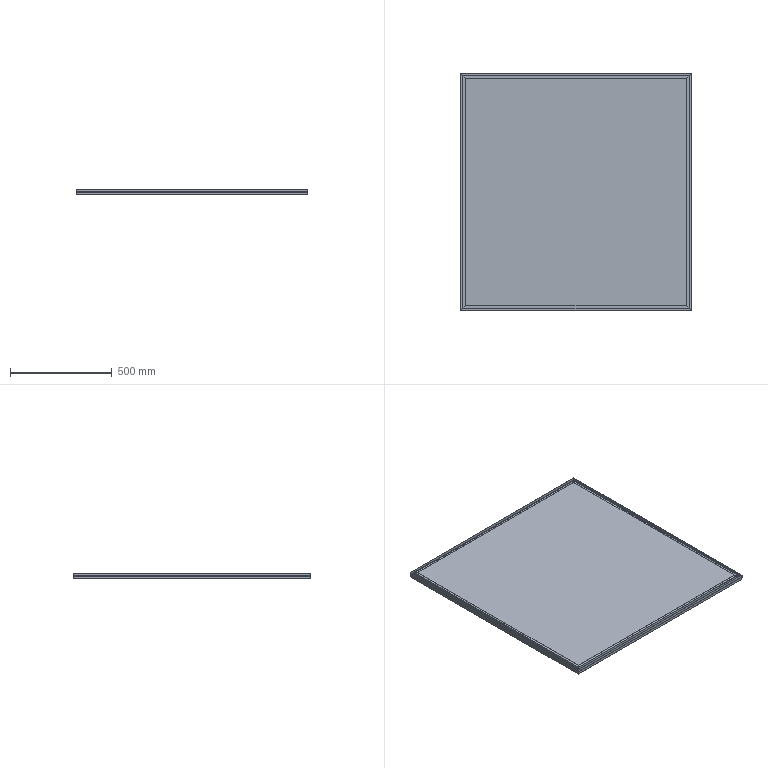Part | 5 solids | 78 faces | box 1140 x 1170 x 27 mm | volume 28599828 mm3 | plane 78